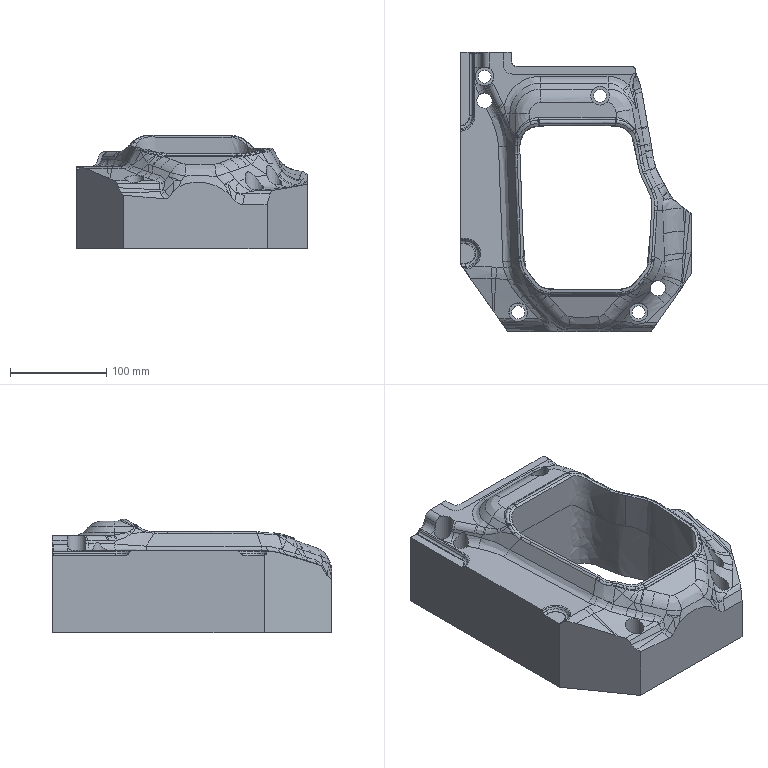Part | NX | features solid 2 | 1 solid | 331 faces | box 240.021 x 290.001 x 118.099 mm | volume 3120336 mm3 | spline 309 | plane 12 | cylinder 10 | commonest cylinder face diameters 13.5 x4 19.5 x4 16 x2